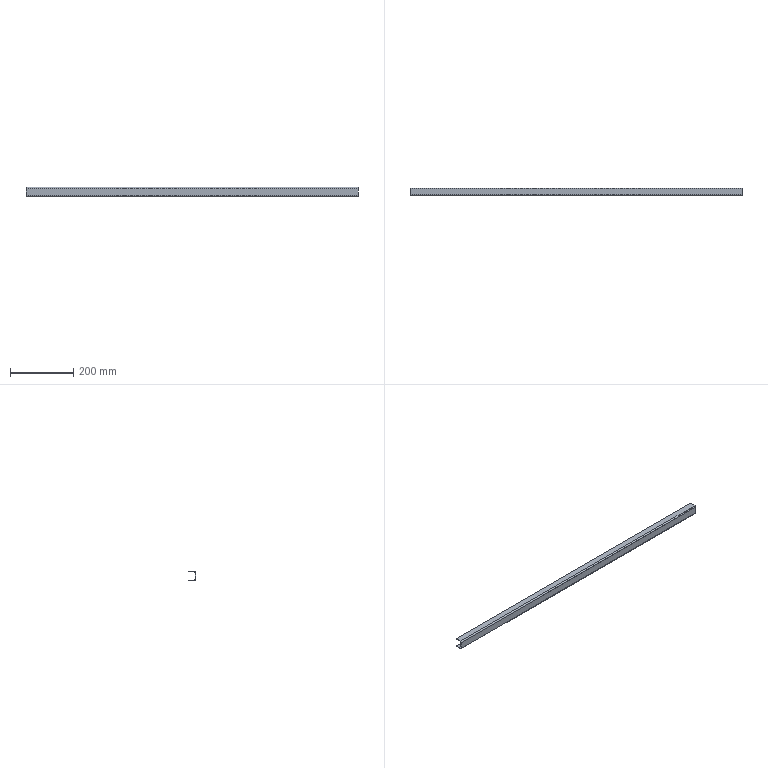Part | NX | features solid 2 | 1 solid | 14 faces | box 1050 x 23 x 30 mm | volume 145792 mm3 | plane 10 | cylinder 4 | commonest cylinder face diameters 4 x2 8 x2
STEP:
#1=CARTESIAN_POINT('',(1138.,-671.,1263.));
#2=VERTEX_POINT('',#1);
#3=CARTESIAN_POINT('',(1138.,-652.,1263.));
#4=VERTEX_POINT('',#3);
#5=CARTESIAN_POINT('',(1138.,-652.,1263.));
#6=DIRECTION('',(0.,1.,0.));
#7=VECTOR('',#6,1000.);
#8=LINE('',#5,#7);
#9=EDGE_CURVE('',#2,#4,#8,.T.);
#10=ORIENTED_EDGE('',*,*,#9,.T.);
#11=CARTESIAN_POINT('',(2188.,-652.,1263.));
#12=VERTEX_POINT('',#11);
#13=CARTESIAN_POINT('',(2188.,-652.,1263.));
#14=DIRECTION('',(-1.,0.,0.));
#15=VECTOR('',#14,1000.);
#16=LINE('',#13,#15);
#17=EDGE_CURVE('',#12,#4,#16,.T.);
#18=ORIENTED_EDGE('',*,*,#17,.F.);
#19=CARTESIAN_POINT('',(2188.,-671.,1263.));
#20=VERTEX_POINT('',#19);
#21=CARTESIAN_POINT('',(2188.,-652.,1263.));
#22=DIRECTION('',(0.,1.,0.));
#23=VECTOR('',#22,1000.);
#24=LINE('',#21,#23);
#25=EDGE_CURVE('',#20,#12,#24,.T.);
#26=ORIENTED_EDGE('',*,*,#25,.F.);
#27=CARTESIAN_POINT('',(2188.,-671.,1263.));
#28=DIRECTION('',(-1.,0.,0.));
#29=VECTOR('',#28,1000.);
#30=LINE('',#27,#29);
#31=EDGE_CURVE('',#20,#2,#30,.T.);
#32=ORIENTED_EDGE('',*,*,#31,.T.);
#33=EDGE_LOOP('',(#10,#18,#26,#32));
#34=FACE_BOUND('',#33,.T.);
#35=CARTESIAN_POINT('',(2188.,-652.,1263.));
#36=DIRECTION('',(0.,0.,1.));
#37=DIRECTION('',(1.,0.,0.));
#38=AXIS2_PLACEMENT_3D('',#35,#36,#37);
#39=PLANE('',#38);
#40=ADVANCED_FACE('',(#34),#39,.F.);
#41=CARTESIAN_POINT('',(1138.,-675.,1267.));
#42=VERTEX_POINT('',#41);
#43=CARTESIAN_POINT('',(1138.,-671.,1267.));
#44=DIRECTION('',(1.,0.,0.));
#45=DIRECTION('',(0.,0.,-1.));
#46=AXIS2_PLACEMENT_3D('',#43,#44,#45);
#47=CIRCLE('',#46,4.);
#48=EDGE_CURVE('',#42,#2,#47,.T.);
#49=ORIENTED_EDGE('',*,*,#48,.T.);
#50=ORIENTED_EDGE('',*,*,#31,.F.);
#51=CARTESIAN_POINT('',(2188.,-675.,1267.));
#52=VERTEX_POINT('',#51);
#53=CARTESIAN_POINT('',(2188.,-671.,1267.));
#54=DIRECTION('',(1.,0.,0.));
#55=DIRECTION('',(0.,0.,-1.));
#56=AXIS2_PLACEMENT_3D('',#53,#54,#55);
#57=CIRCLE('',#56,4.);
#58=EDGE_CURVE('',#52,#20,#57,.T.);
#59=ORIENTED_EDGE('',*,*,#58,.F.);
#60=CARTESIAN_POINT('',(2188.,-675.,1267.));
#61=DIRECTION('',(-1.,0.,0.));
#62=VECTOR('',#61,1000.);
#63=LINE('',#60,#62);
#64=EDGE_CURVE('',#52,#42,#63,.T.);
#65=ORIENTED_EDGE('',*,*,#64,.T.);
#66=EDGE_LOOP('',(#49,#50,#59,#65));
#67=FACE_BOUND('',#66,.T.);
#68=CARTESIAN_POINT('',(2188.,-671.,1267.));
#69=DIRECTION('',(-1.,0.,0.));
#70=DIRECTION('',(0.,0.,-1.));
#71=AXIS2_PLACEMENT_3D('',#68,#69,#70);
#72=CYLINDRICAL_SURFACE('',#71,4.);
#73=ADVANCED_FACE('',(#67),#72,.T.);
#74=CARTESIAN_POINT('',(1138.,-675.,1289.));
#75=VERTEX_POINT('',#74);
#76=CARTESIAN_POINT('',(1138.,-675.,1265.));
#77=DIRECTION('',(0.,0.,-1.));
#78=VECTOR('',#77,1000.);
#79=LINE('',#76,#78);
#80=EDGE_CURVE('',#75,#42,#79,.T.);
#81=ORIENTED_EDGE('',*,*,#80,.T.);
#82=ORIENTED_EDGE('',*,*,#64,.F.);
#83=CARTESIAN_POINT('',(2188.,-675.,1289.));
#84=VERTEX_POINT('',#83);
#85=CARTESIAN_POINT('',(2188.,-675.,1265.));
#86=DIRECTION('',(0.,0.,-1.));
#87=VECTOR('',#86,1000.);
#88=LINE('',#85,#87);
#89=EDGE_CURVE('',#84,#52,#88,.T.);
#90=ORIENTED_EDGE('',*,*,#89,.F.);
#91=CARTESIAN_POINT('',(2188.,-675.,1289.));
#92=DIRECTION('',(-1.,0.,0.));
#93=VECTOR('',#92,1000.);
#94=LINE('',#91,#93);
#95=EDGE_CURVE('',#84,#75,#94,.T.);
#96=ORIENTED_EDGE('',*,*,#95,.T.);
#97=EDGE_LOOP('',(#81,#82,#90,#96));
#98=FACE_BOUND('',#97,.T.);
#99=CARTESIAN_POINT('',(2188.,-675.,1265.));
#100=DIRECTION('',(0.,1.,0.));
#101=DIRECTION('',(0.,0.,-1.));
#102=AXIS2_PLACEMENT_3D('',#99,#100,#101);
#103=PLANE('',#102);
#104=ADVANCED_FACE('',(#98),#103,.F.);
#105=CARTESIAN_POINT('',(1138.,-671.,1293.));
#106=VERTEX_POINT('',#105);
#107=CARTESIAN_POINT('',(1138.,-671.,1289.));
#108=DIRECTION('',(1.,0.,0.));
#109=DIRECTION('',(0.,0.,-1.));
#110=AXIS2_PLACEMENT_3D('',#107,#108,#109);
#111=CIRCLE('',#110,4.);
#112=EDGE_CURVE('',#106,#75,#111,.T.);
#113=ORIENTED_EDGE('',*,*,#112,.T.);
#114=ORIENTED_EDGE('',*,*,#95,.F.);
#115=CARTESIAN_POINT('',(2188.,-671.,1293.));
#116=VERTEX_POINT('',#115);
#117=CARTESIAN_POINT('',(2188.,-671.,1289.));
#118=DIRECTION('',(1.,0.,0.));
#119=DIRECTION('',(0.,0.,-1.));
#120=AXIS2_PLACEMENT_3D('',#117,#118,#119);
#121=CIRCLE('',#120,4.);
#122=EDGE_CURVE('',#116,#84,#121,.T.);
#123=ORIENTED_EDGE('',*,*,#122,.F.);
#124=CARTESIAN_POINT('',(2188.,-671.,1293.));
#125=DIRECTION('',(-1.,0.,0.));
#126=VECTOR('',#125,1000.);
#127=LINE('',#124,#126);
#128=EDGE_CURVE('',#116,#106,#127,.T.);
#129=ORIENTED_EDGE('',*,*,#128,.T.);
#130=EDGE_LOOP('',(#113,#114,#123,#129));
#131=FACE_BOUND('',#130,.T.);
#132=CARTESIAN_POINT('',(2188.,-671.,1289.));
#133=DIRECTION('',(-1.,0.,0.));
#134=DIRECTION('',(0.,0.,-1.));
#135=AXIS2_PLACEMENT_3D('',#132,#133,#134);
#136=CYLINDRICAL_SURFACE('',#135,4.);
#137=ADVANCED_FACE('',(#131),#136,.T.);
#138=CARTESIAN_POINT('',(1138.,-652.,1293.));
#139=VERTEX_POINT('',#138);
#140=CARTESIAN_POINT('',(1138.,-673.,1293.));
#141=DIRECTION('',(0.,-1.,0.));
#142=VECTOR('',#141,1000.);
#143=LINE('',#140,#142);
#144=EDGE_CURVE('',#139,#106,#143,.T.);
#145=ORIENTED_EDGE('',*,*,#144,.T.);
#146=ORIENTED_EDGE('',*,*,#128,.F.);
#147=CARTESIAN_POINT('',(2188.,-652.,1293.));
#148=VERTEX_POINT('',#147);
#149=CARTESIAN_POINT('',(2188.,-673.,1293.));
#150=DIRECTION('',(0.,-1.,0.));
#151=VECTOR('',#150,1000.);
#152=LINE('',#149,#151);
#153=EDGE_CURVE('',#148,#116,#152,.T.);
#154=ORIENTED_EDGE('',*,*,#153,.F.);
#155=CARTESIAN_POINT('',(2188.,-652.,1293.));
#156=DIRECTION('',(-1.,0.,0.));
#157=VECTOR('',#156,1000.);
#158=LINE('',#155,#157);
#159=EDGE_CURVE('',#148,#139,#158,.T.);
#160=ORIENTED_EDGE('',*,*,#159,.T.);
#161=EDGE_LOOP('',(#145,#146,#154,#160));
#162=FACE_BOUND('',#161,.T.);
#163=CARTESIAN_POINT('',(2188.,-673.,1293.));
#164=DIRECTION('',(0.,0.,-1.));
#165=DIRECTION('',(0.,-1.,0.));
#166=AXIS2_PLACEMENT_3D('',#163,#164,#165);
#167=PLANE('',#166);
#168=ADVANCED_FACE('',(#162),#167,.F.);
#169=CARTESIAN_POINT('',(1138.,-671.,1265.));
#170=VERTEX_POINT('',#169);
#171=CARTESIAN_POINT('',(1138.,-652.,1265.));
#172=VERTEX_POINT('',#171);
#173=CARTESIAN_POINT('',(1138.,-652.,1265.));
#174=DIRECTION('',(0.,1.,0.));
#175=VECTOR('',#174,1000.);
#176=LINE('',#173,#175);
#177=EDGE_CURVE('',#170,#172,#176,.T.);
#178=ORIENTED_EDGE('',*,*,#177,.F.);
#179=CARTESIAN_POINT('',(2188.,-671.,1265.));
#180=VERTEX_POINT('',#179);
#181=CARTESIAN_POINT('',(2188.,-671.,1265.));
#182=DIRECTION('',(-1.,0.,0.));
#183=VECTOR('',#182,1000.);
#184=LINE('',#181,#183);
#185=EDGE_CURVE('',#180,#170,#184,.T.);
#186=ORIENTED_EDGE('',*,*,#185,.F.);
#187=CARTESIAN_POINT('',(2188.,-652.,1265.));
#188=VERTEX_POINT('',#187);
#189=CARTESIAN_POINT('',(2188.,-652.,1265.));
#190=DIRECTION('',(0.,1.,0.));
#191=VECTOR('',#190,1000.);
#192=LINE('',#189,#191);
#193=EDGE_CURVE('',#180,#188,#192,.T.);
#194=ORIENTED_EDGE('',*,*,#193,.T.);
#195=CARTESIAN_POINT('',(2188.,-652.,1265.));
#196=DIRECTION('',(-1.,0.,0.));
#197=VECTOR('',#196,1000.);
#198=LINE('',#195,#197);
#199=EDGE_CURVE('',#188,#172,#198,.T.);
#200=ORIENTED_EDGE('',*,*,#199,.T.);
#201=EDGE_LOOP('',(#178,#186,#194,#200));
#202=FACE_BOUND('',#201,.T.);
#203=CARTESIAN_POINT('',(2188.,-652.,1265.));
#204=DIRECTION('',(0.,0.,1.));
#205=DIRECTION('',(1.,0.,0.));
#206=AXIS2_PLACEMENT_3D('',#203,#204,#205);
#207=PLANE('',#206);
#208=ADVANCED_FACE('',(#202),#207,.T.);
#209=CARTESIAN_POINT('',(1138.,-673.,1267.));
#210=VERTEX_POINT('',#209);
#211=CARTESIAN_POINT('',(1138.,-671.,1267.));
#212=DIRECTION('',(1.,0.,0.));
#213=DIRECTION('',(0.,0.,-1.));
#214=AXIS2_PLACEMENT_3D('',#211,#212,#213);
#215=CIRCLE('',#214,2.);
#216=EDGE_CURVE('',#210,#170,#215,.T.);
#217=ORIENTED_EDGE('',*,*,#216,.F.);
#218=CARTESIAN_POINT('',(2188.,-673.,1267.));
#219=VERTEX_POINT('',#218);
#220=CARTESIAN_POINT('',(2188.,-673.,1267.));
#221=DIRECTION('',(-1.,0.,0.));
#222=VECTOR('',#221,1000.);
#223=LINE('',#220,#222);
#224=EDGE_CURVE('',#219,#210,#223,.T.);
#225=ORIENTED_EDGE('',*,*,#224,.F.);
#226=CARTESIAN_POINT('',(2188.,-671.,1267.));
#227=DIRECTION('',(1.,0.,0.));
#228=DIRECTION('',(0.,0.,-1.));
#229=AXIS2_PLACEMENT_3D('',#226,#227,#228);
#230=CIRCLE('',#229,2.);
#231=EDGE_CURVE('',#219,#180,#230,.T.);
#232=ORIENTED_EDGE('',*,*,#231,.T.);
#233=ORIENTED_EDGE('',*,*,#185,.T.);
#234=EDGE_LOOP('',(#217,#225,#232,#233));
#235=FACE_BOUND('',#234,.T.);
#236=CARTESIAN_POINT('',(2188.,-671.,1267.));
#237=DIRECTION('',(-1.,0.,0.));
#238=DIRECTION('',(0.,0.,-1.));
#239=AXIS2_PLACEMENT_3D('',#236,#237,#238);
#240=CYLINDRICAL_SURFACE('',#239,2.);
#241=ADVANCED_FACE('',(#235),#240,.F.);
#242=CARTESIAN_POINT('',(1138.,-673.,1289.));
#243=VERTEX_POINT('',#242);
#244=CARTESIAN_POINT('',(1138.,-673.,1265.));
#245=DIRECTION('',(0.,0.,-1.));
#246=VECTOR('',#245,1000.);
#247=LINE('',#244,#246);
#248=EDGE_CURVE('',#243,#210,#247,.T.);
#249=ORIENTED_EDGE('',*,*,#248,.F.);
#250=CARTESIAN_POINT('',(2188.,-673.,1289.));
#251=VERTEX_POINT('',#250);
#252=CARTESIAN_POINT('',(2188.,-673.,1289.));
#253=DIRECTION('',(-1.,0.,0.));
#254=VECTOR('',#253,1000.);
#255=LINE('',#252,#254);
#256=EDGE_CURVE('',#251,#243,#255,.T.);
#257=ORIENTED_EDGE('',*,*,#256,.F.);
#258=CARTESIAN_POINT('',(2188.,-673.,1265.));
#259=DIRECTION('',(0.,0.,-1.));
#260=VECTOR('',#259,1000.);
#261=LINE('',#258,#260);
#262=EDGE_CURVE('',#251,#219,#261,.T.);
#263=ORIENTED_EDGE('',*,*,#262,.T.);
#264=ORIENTED_EDGE('',*,*,#224,.T.);
#265=EDGE_LOOP('',(#249,#257,#263,#264));
#266=FACE_BOUND('',#265,.T.);
#267=CARTESIAN_POINT('',(2188.,-673.,1265.));
#268=DIRECTION('',(0.,1.,0.));
#269=DIRECTION('',(0.,0.,-1.));
#270=AXIS2_PLACEMENT_3D('',#267,#268,#269);
#271=PLANE('',#270);
#272=ADVANCED_FACE('',(#266),#271,.T.);
#273=CARTESIAN_POINT('',(1138.,-671.,1291.));
#274=VERTEX_POINT('',#273);
#275=CARTESIAN_POINT('',(1138.,-671.,1289.));
#276=DIRECTION('',(1.,0.,0.));
#277=DIRECTION('',(0.,0.,-1.));
#278=AXIS2_PLACEMENT_3D('',#275,#276,#277);
#279=CIRCLE('',#278,2.);
#280=EDGE_CURVE('',#274,#243,#279,.T.);
#281=ORIENTED_EDGE('',*,*,#280,.F.);
#282=CARTESIAN_POINT('',(2188.,-671.,1291.));
#283=VERTEX_POINT('',#282);
#284=CARTESIAN_POINT('',(2188.,-671.,1291.));
#285=DIRECTION('',(-1.,0.,0.));
#286=VECTOR('',#285,1000.);
#287=LINE('',#284,#286);
#288=EDGE_CURVE('',#283,#274,#287,.T.);
#289=ORIENTED_EDGE('',*,*,#288,.F.);
#290=CARTESIAN_POINT('',(2188.,-671.,1289.));
#291=DIRECTION('',(1.,0.,0.));
#292=DIRECTION('',(0.,0.,-1.));
#293=AXIS2_PLACEMENT_3D('',#290,#291,#292);
#294=CIRCLE('',#293,2.);
#295=EDGE_CURVE('',#283,#251,#294,.T.);
#296=ORIENTED_EDGE('',*,*,#295,.T.);
#297=ORIENTED_EDGE('',*,*,#256,.T.);
#298=EDGE_LOOP('',(#281,#289,#296,#297));
#299=FACE_BOUND('',#298,.T.);
#300=CARTESIAN_POINT('',(2188.,-671.,1289.));
#301=DIRECTION('',(-1.,0.,0.));
#302=DIRECTION('',(0.,0.,-1.));
#303=AXIS2_PLACEMENT_3D('',#300,#301,#302);
#304=CYLINDRICAL_SURFACE('',#303,2.);
#305=ADVANCED_FACE('',(#299),#304,.F.);
#306=CARTESIAN_POINT('',(1138.,-652.,1291.));
#307=VERTEX_POINT('',#306);
#308=CARTESIAN_POINT('',(1138.,-673.,1291.));
#309=DIRECTION('',(0.,-1.,0.));
#310=VECTOR('',#309,1000.);
#311=LINE('',#308,#310);
#312=EDGE_CURVE('',#307,#274,#311,.T.);
#313=ORIENTED_EDGE('',*,*,#312,.F.);
#314=CARTESIAN_POINT('',(2188.,-652.,1291.));
#315=VERTEX_POINT('',#314);
#316=CARTESIAN_POINT('',(2188.,-652.,1291.));
#317=DIRECTION('',(-1.,0.,0.));
#318=VECTOR('',#317,1000.);
#319=LINE('',#316,#318);
#320=EDGE_CURVE('',#315,#307,#319,.T.);
#321=ORIENTED_EDGE('',*,*,#320,.F.);
#322=CARTESIAN_POINT('',(2188.,-673.,1291.));
#323=DIRECTION('',(0.,-1.,0.));
#324=VECTOR('',#323,1000.);
#325=LINE('',#322,#324);
#326=EDGE_CURVE('',#315,#283,#325,.T.);
#327=ORIENTED_EDGE('',*,*,#326,.T.);
#328=ORIENTED_EDGE('',*,*,#288,.T.);
#329=EDGE_LOOP('',(#313,#321,#327,#328));
#330=FACE_BOUND('',#329,.T.);
#331=CARTESIAN_POINT('',(2188.,-673.,1291.));
#332=DIRECTION('',(0.,0.,-1.));
#333=DIRECTION('',(0.,-1.,0.));
#334=AXIS2_PLACEMENT_3D('',#331,#332,#333);
#335=PLANE('',#334);
#336=ADVANCED_FACE('',(#330),#335,.T.);
#337=ORIENTED_EDGE('',*,*,#159,.F.);
#338=CARTESIAN_POINT('',(2188.,-652.,1291.));
#339=DIRECTION('',(0.,0.,-1.));
#340=VECTOR('',#339,1000.);
#341=LINE('',#338,#340);
#342=EDGE_CURVE('',#148,#315,#341,.T.);
#343=ORIENTED_EDGE('',*,*,#342,.T.);
#344=ORIENTED_EDGE('',*,*,#320,.T.);
#345=CARTESIAN_POINT('',(1138.,-652.,1291.));
#346=DIRECTION('',(0.,0.,-1.));
#347=VECTOR('',#346,1000.);
#348=LINE('',#345,#347);
#349=EDGE_CURVE('',#139,#307,#348,.T.);
#350=ORIENTED_EDGE('',*,*,#349,.F.);
#351=EDGE_LOOP('',(#337,#343,#344,#350));
#352=FACE_BOUND('',#351,.T.);
#353=CARTESIAN_POINT('',(2188.,-652.,1291.));
#354=DIRECTION('',(0.,-1.,0.));
#355=DIRECTION('',(-1.,0.,0.));
#356=AXIS2_PLACEMENT_3D('',#353,#354,#355);
#357=PLANE('',#356);
#358=ADVANCED_FACE('',(#352),#357,.F.);
#359=ORIENTED_EDGE('',*,*,#312,.T.);
#360=ORIENTED_EDGE('',*,*,#280,.T.);
#361=ORIENTED_EDGE('',*,*,#248,.T.);
#362=ORIENTED_EDGE('',*,*,#216,.T.);
#363=ORIENTED_EDGE('',*,*,#177,.T.);
#364=CARTESIAN_POINT('',(1138.,-652.,1265.));
#365=DIRECTION('',(0.,0.,1.));
#366=VECTOR('',#365,1000.);
#367=LINE('',#364,#366);
#368=EDGE_CURVE('',#4,#172,#367,.T.);
#369=ORIENTED_EDGE('',*,*,#368,.F.);
#370=ORIENTED_EDGE('',*,*,#9,.F.);
#371=ORIENTED_EDGE('',*,*,#48,.F.);
#372=ORIENTED_EDGE('',*,*,#80,.F.);
#373=ORIENTED_EDGE('',*,*,#112,.F.);
#374=ORIENTED_EDGE('',*,*,#144,.F.);
#375=ORIENTED_EDGE('',*,*,#349,.T.);
#376=EDGE_LOOP('',(#359,#360,#361,#362,#363,#369,#370,#371,#372,#373,#374,#375));
#377=FACE_BOUND('',#376,.T.);
#378=CARTESIAN_POINT('',(1138.,-673.,1291.));
#379=DIRECTION('',(1.,0.,0.));
#380=DIRECTION('',(0.,0.,1.));
#381=AXIS2_PLACEMENT_3D('',#378,#379,#380);
#382=PLANE('',#381);
#383=ADVANCED_FACE('',(#377),#382,.F.);
#384=CARTESIAN_POINT('',(2188.,-652.,1265.));
#385=DIRECTION('',(0.,0.,1.));
#386=VECTOR('',#385,1000.);
#387=LINE('',#384,#386);
#388=EDGE_CURVE('',#12,#188,#387,.T.);
#389=ORIENTED_EDGE('',*,*,#388,.F.);
#390=ORIENTED_EDGE('',*,*,#17,.T.);
#391=ORIENTED_EDGE('',*,*,#368,.T.);
#392=ORIENTED_EDGE('',*,*,#199,.F.);
#393=EDGE_LOOP('',(#389,#390,#391,#392));
#394=FACE_BOUND('',#393,.T.);
#395=CARTESIAN_POINT('',(2188.,-652.,1265.));
#396=DIRECTION('',(0.,1.,0.));
#397=DIRECTION('',(0.,0.,-1.));
#398=AXIS2_PLACEMENT_3D('',#395,#396,#397);
#399=PLANE('',#398);
#400=ADVANCED_FACE('',(#394),#399,.T.);
#401=ORIENTED_EDGE('',*,*,#193,.F.);
#402=ORIENTED_EDGE('',*,*,#231,.F.);
#403=ORIENTED_EDGE('',*,*,#262,.F.);
#404=ORIENTED_EDGE('',*,*,#295,.F.);
#405=ORIENTED_EDGE('',*,*,#326,.F.);
#406=ORIENTED_EDGE('',*,*,#342,.F.);
#407=ORIENTED_EDGE('',*,*,#153,.T.);
#408=ORIENTED_EDGE('',*,*,#122,.T.);
#409=ORIENTED_EDGE('',*,*,#89,.T.);
#410=ORIENTED_EDGE('',*,*,#58,.T.);
#411=ORIENTED_EDGE('',*,*,#25,.T.);
#412=ORIENTED_EDGE('',*,*,#388,.T.);
#413=EDGE_LOOP('',(#401,#402,#403,#404,#405,#406,#407,#408,#409,#410,#411,#412));
#414=FACE_BOUND('',#413,.T.);
#415=CARTESIAN_POINT('',(2188.,-652.,1265.));
#416=DIRECTION('',(1.,0.,0.));
#417=DIRECTION('',(0.,0.,1.));
#418=AXIS2_PLACEMENT_3D('',#415,#416,#417);
#419=PLANE('',#418);
#420=ADVANCED_FACE('',(#414),#419,.T.);
#421=CLOSED_SHELL('',(#40,#73,#104,#137,#168,#208,#241,#272,#305,#336,#358,#383,#400,#420));
#422=MANIFOLD_SOLID_BREP('',#421);
#423=(LENGTH_UNIT()NAMED_UNIT(*)SI_UNIT(.MILLI.,.METRE.));
#424=UNCERTAINTY_MEASURE_WITH_UNIT(LENGTH_MEASURE(0.00001),#423,'','');
#425=(NAMED_UNIT(*)PLANE_ANGLE_UNIT()SI_UNIT($,.RADIAN.));
#426=(NAMED_UNIT(*)SI_UNIT($,.STERADIAN.)SOLID_ANGLE_UNIT());
#427=(GEOMETRIC_REPRESENTATION_CONTEXT(3)GLOBAL_UNCERTAINTY_ASSIGNED_CONTEXT((#424))GLOBAL_UNIT_ASSIGNED_CONTEXT((#423,#425,#426))REPRESENTATION_CONTEXT('',''));
#428=ADVANCED_BREP_SHAPE_REPRESENTATION('',(#422),#427);